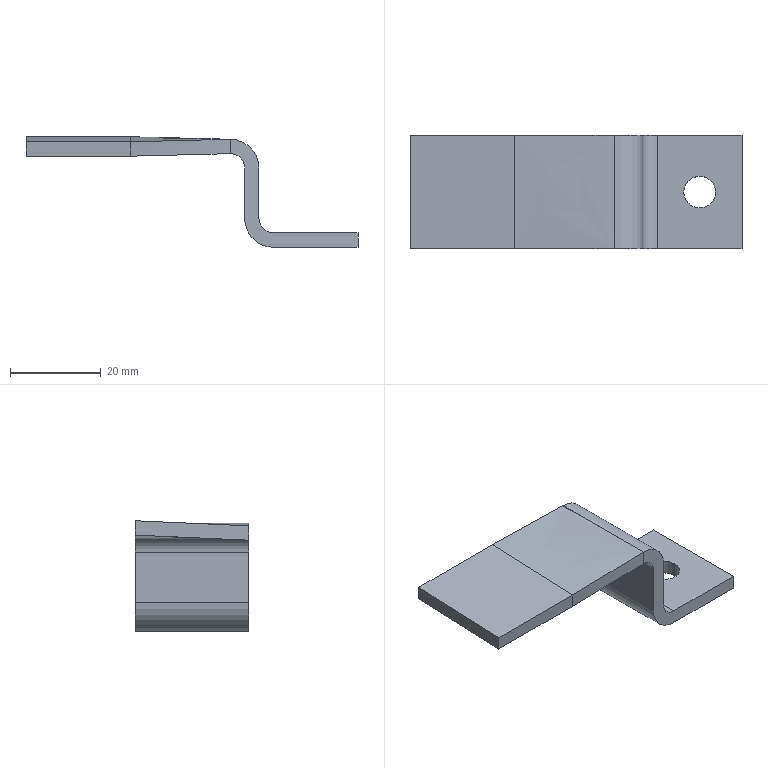Part | SolidWorks | features BaseBody 1 | 1 solid | 24 faces | box 73.18 x 25.116 x 24.356 mm | volume 6989 mm3 | plane 14 | cylinder 6 | spline 4 | commonest cylinder face diameters 6.34 x2 7 x2 12.68 x2
STEP:
#1=CARTESIAN_POINT('',(8.393,12.209,3.17));
#2=VERTEX_POINT('',#1);
#3=CARTESIAN_POINT('',(1.393,12.209,3.17));
#4=VERTEX_POINT('',#3);
#5=CARTESIAN_POINT('',(4.893,12.209,3.17));
#6=DIRECTION('',(0.,0.,-1.));
#7=DIRECTION('',(-1.,0.,0.));
#8=AXIS2_PLACEMENT_3D('',#5,#6,#7);
#9=CIRCLE('',#8,3.5);
#10=EDGE_CURVE('',#2,#4,#9,.T.);
#11=ORIENTED_EDGE('',*,*,#10,.F.);
#12=CARTESIAN_POINT('',(8.393,12.209,0.));
#13=VERTEX_POINT('',#12);
#14=CARTESIAN_POINT('',(8.393,12.209,81.122));
#15=DIRECTION('',(0.,0.,-1.));
#16=VECTOR('',#15,1000.);
#17=LINE('',#14,#16);
#18=EDGE_CURVE('',#2,#13,#17,.T.);
#19=ORIENTED_EDGE('',*,*,#18,.T.);
#20=CARTESIAN_POINT('',(1.393,12.209,0.));
#21=VERTEX_POINT('',#20);
#22=CARTESIAN_POINT('',(4.893,12.209,0.));
#23=DIRECTION('',(0.,0.,-1.));
#24=DIRECTION('',(-1.,0.,0.));
#25=AXIS2_PLACEMENT_3D('',#22,#23,#24);
#26=CIRCLE('',#25,3.5);
#27=EDGE_CURVE('',#13,#21,#26,.T.);
#28=ORIENTED_EDGE('',*,*,#27,.T.);
#29=CARTESIAN_POINT('',(1.393,12.209,81.122));
#30=DIRECTION('',(0.,0.,-1.));
#31=VECTOR('',#30,1000.);
#32=LINE('',#29,#31);
#33=EDGE_CURVE('',#4,#21,#32,.T.);
#34=ORIENTED_EDGE('',*,*,#33,.F.);
#35=EDGE_LOOP('',(#11,#19,#28,#34));
#36=FACE_OUTER_BOUND('',#35,.T.);
#37=CARTESIAN_POINT('',(4.893,12.209,81.122));
#38=DIRECTION('',(0.,0.,-1.));
#39=DIRECTION('',(-1.,0.,0.));
#40=AXIS2_PLACEMENT_3D('',#37,#38,#39);
#41=CYLINDRICAL_SURFACE('',#40,3.5);
#42=ADVANCED_FACE('',(#36),#41,.F.);
#43=CARTESIAN_POINT('',(-35.957,24.767,21.189));
#44=VERTEX_POINT('',#43);
#45=CARTESIAN_POINT('',(-35.957,-0.2082,20.074));
#46=VERTEX_POINT('',#45);
#47=CARTESIAN_POINT('',(-35.957,-0.2082,20.074));
#48=DIRECTION('',(0.,-0.999,-0.04458));
#49=VECTOR('',#48,1000.);
#50=LINE('',#47,#49);
#51=EDGE_CURVE('',#44,#46,#50,.T.);
#52=ORIENTED_EDGE('',*,*,#51,.T.);
#53=CARTESIAN_POINT('',(-58.957,-0.2082,20.074));
#54=VERTEX_POINT('',#53);
#55=CARTESIAN_POINT('',(-35.957,-0.2082,20.074));
#56=DIRECTION('',(-1.,0.,0.));
#57=VECTOR('',#56,1000.);
#58=LINE('',#55,#57);
#59=EDGE_CURVE('',#46,#54,#58,.T.);
#60=ORIENTED_EDGE('',*,*,#59,.T.);
#61=CARTESIAN_POINT('',(-58.957,24.767,21.189));
#62=VERTEX_POINT('',#61);
#63=CARTESIAN_POINT('',(-58.957,-0.2082,20.074));
#64=DIRECTION('',(0.,0.999,0.04458));
#65=VECTOR('',#64,1000.);
#66=LINE('',#63,#65);
#67=EDGE_CURVE('',#54,#62,#66,.T.);
#68=ORIENTED_EDGE('',*,*,#67,.T.);
#69=CARTESIAN_POINT('',(-35.957,24.767,21.189));
#70=DIRECTION('',(1.,0.,0.));
#71=VECTOR('',#70,1000.);
#72=LINE('',#69,#71);
#73=EDGE_CURVE('',#62,#44,#72,.T.);
#74=ORIENTED_EDGE('',*,*,#73,.T.);
#75=EDGE_LOOP('',(#52,#60,#68,#74));
#76=FACE_OUTER_BOUND('',#75,.T.);
#77=CARTESIAN_POINT('',(-35.957,-0.2082,20.074));
#78=DIRECTION('',(0.,0.04458,-0.999));
#79=DIRECTION('',(0.,0.999,0.04458));
#80=AXIS2_PLACEMENT_3D('',#77,#78,#79);
#81=PLANE('',#80);
#82=ADVANCED_FACE('',(#76),#81,.T.);
#83=CARTESIAN_POINT('',(-35.957,-0.3495,23.241));
#84=VERTEX_POINT('',#83);
#85=CARTESIAN_POINT('',(-35.957,-0.2788,21.658));
#86=DIRECTION('',(0.,0.04458,-0.999));
#87=VECTOR('',#86,1000.);
#88=LINE('',#85,#87);
#89=EDGE_CURVE('',#84,#46,#88,.T.);
#90=ORIENTED_EDGE('',*,*,#89,.F.);
#91=CARTESIAN_POINT('',(-58.957,-0.3495,23.241));
#92=VERTEX_POINT('',#91);
#93=CARTESIAN_POINT('',(-35.957,-0.3495,23.241));
#94=DIRECTION('',(-1.,0.,0.));
#95=VECTOR('',#94,1000.);
#96=LINE('',#93,#95);
#97=EDGE_CURVE('',#84,#92,#96,.T.);
#98=ORIENTED_EDGE('',*,*,#97,.T.);
#99=CARTESIAN_POINT('',(-58.957,-0.3495,23.241));
#100=DIRECTION('',(0.,0.04458,-0.999));
#101=VECTOR('',#100,1000.);
#102=LINE('',#99,#101);
#103=EDGE_CURVE('',#92,#54,#102,.T.);
#104=ORIENTED_EDGE('',*,*,#103,.T.);
#105=ORIENTED_EDGE('',*,*,#59,.F.);
#106=EDGE_LOOP('',(#90,#98,#104,#105));
#107=FACE_OUTER_BOUND('',#106,.T.);
#108=CARTESIAN_POINT('',(-35.957,-0.3495,23.241));
#109=DIRECTION('',(0.,-0.999,-0.04458));
#110=DIRECTION('',(0.,0.04458,-0.999));
#111=AXIS2_PLACEMENT_3D('',#108,#109,#110);
#112=PLANE('',#111);
#113=ADVANCED_FACE('',(#107),#112,.T.);
#114=CARTESIAN_POINT('',(-13.957,24.709,20.63));
#115=VERTEX_POINT('',#114);
#116=CARTESIAN_POINT('',(-13.957,-0.2913,20.63));
#117=VERTEX_POINT('',#116);
#118=CARTESIAN_POINT('',(-13.957,12.209,20.63));
#119=DIRECTION('',(0.,-1.,0.));
#120=VECTOR('',#119,1000.);
#121=LINE('',#118,#120);
#122=EDGE_CURVE('',#115,#117,#121,.T.);
#123=ORIENTED_EDGE('',*,*,#122,.T.);
#124=CARTESIAN_POINT('',(-13.957,-0.2913,20.63));
#125=CARTESIAN_POINT('',(-21.29,-0.2677,20.444));
#126=CARTESIAN_POINT('',(-28.623,-0.24,20.259));
#127=CARTESIAN_POINT('',(-35.957,-0.2082,20.074));
#128=B_SPLINE_CURVE_WITH_KNOTS('',3,(#124,#125,#126,#127),.UNSPECIFIED.,.F.,.F.,(4,4),(0.,0.04459),.UNSPECIFIED.);
#129=EDGE_CURVE('',#117,#46,#128,.T.);
#130=ORIENTED_EDGE('',*,*,#129,.T.);
#131=ORIENTED_EDGE('',*,*,#51,.F.);
#132=CARTESIAN_POINT('',(-35.957,24.767,21.189));
#133=CARTESIAN_POINT('',(-28.623,24.752,21.002));
#134=CARTESIAN_POINT('',(-21.29,24.732,20.816));
#135=CARTESIAN_POINT('',(-13.957,24.709,20.63));
#136=B_SPLINE_CURVE_WITH_KNOTS('',3,(#132,#133,#134,#135),.UNSPECIFIED.,.F.,.F.,(4,4),(0.,0.04459),.UNSPECIFIED.);
#137=EDGE_CURVE('',#44,#115,#136,.T.);
#138=ORIENTED_EDGE('',*,*,#137,.T.);
#139=EDGE_LOOP('',(#123,#130,#131,#138));
#140=FACE_OUTER_BOUND('',#139,.T.);
#141=CARTESIAN_POINT('',(-13.957,24.709,20.63));
#142=CARTESIAN_POINT('',(-21.29,24.732,20.816));
#143=CARTESIAN_POINT('',(-28.623,24.752,21.002));
#144=CARTESIAN_POINT('',(-35.957,24.767,21.189));
#145=CARTESIAN_POINT('',(-13.957,16.375,20.63));
#146=CARTESIAN_POINT('',(-21.29,16.399,20.692));
#147=CARTESIAN_POINT('',(-28.623,16.421,20.754));
#148=CARTESIAN_POINT('',(-35.957,16.442,20.817));
#149=CARTESIAN_POINT('',(-13.957,8.042,20.63));
#150=CARTESIAN_POINT('',(-21.29,8.066,20.568));
#151=CARTESIAN_POINT('',(-28.623,8.091,20.507));
#152=CARTESIAN_POINT('',(-35.957,8.117,20.446));
#153=CARTESIAN_POINT('',(-13.957,-0.2913,20.63));
#154=CARTESIAN_POINT('',(-21.29,-0.2677,20.444));
#155=CARTESIAN_POINT('',(-28.623,-0.24,20.259));
#156=CARTESIAN_POINT('',(-35.957,-0.2082,20.074));
#157=B_SPLINE_SURFACE_WITH_KNOTS('',3,3,((#141,#142,#143,#144),(#145,#146,#147,#148),(#149,#150,#151,#152),(#153,#154,#155,#156)),.UNSPECIFIED.,.F.,.F.,.F.,(4,4),(4,4),(0.,2.5),(0.,0.04459),.UNSPECIFIED.);
#158=ADVANCED_FACE('',(#140),#157,.T.);
#159=CARTESIAN_POINT('',(-35.957,24.626,24.356));
#160=VERTEX_POINT('',#159);
#161=CARTESIAN_POINT('',(-35.957,24.767,21.189));
#162=DIRECTION('',(0.,0.04458,-0.999));
#163=VECTOR('',#162,1000.);
#164=LINE('',#161,#163);
#165=EDGE_CURVE('',#160,#44,#164,.T.);
#166=ORIENTED_EDGE('',*,*,#165,.T.);
#167=ORIENTED_EDGE('',*,*,#73,.F.);
#168=CARTESIAN_POINT('',(-58.957,24.626,24.356));
#169=VERTEX_POINT('',#168);
#170=CARTESIAN_POINT('',(-58.957,24.767,21.189));
#171=DIRECTION('',(0.,-0.04458,0.999));
#172=VECTOR('',#171,1000.);
#173=LINE('',#170,#172);
#174=EDGE_CURVE('',#62,#169,#173,.T.);
#175=ORIENTED_EDGE('',*,*,#174,.T.);
#176=CARTESIAN_POINT('',(-35.957,24.626,24.356));
#177=DIRECTION('',(1.,0.,0.));
#178=VECTOR('',#177,1000.);
#179=LINE('',#176,#178);
#180=EDGE_CURVE('',#169,#160,#179,.T.);
#181=ORIENTED_EDGE('',*,*,#180,.T.);
#182=EDGE_LOOP('',(#166,#167,#175,#181));
#183=FACE_OUTER_BOUND('',#182,.T.);
#184=CARTESIAN_POINT('',(-35.957,24.767,21.189));
#185=DIRECTION('',(0.,0.999,0.04458));
#186=DIRECTION('',(0.,-0.04458,0.999));
#187=AXIS2_PLACEMENT_3D('',#184,#185,#186);
#188=PLANE('',#187);
#189=ADVANCED_FACE('',(#183),#188,.T.);
#190=CARTESIAN_POINT('',(-58.957,24.626,24.356));
#191=DIRECTION('',(0.,-0.999,-0.04458));
#192=VECTOR('',#191,1000.);
#193=LINE('',#190,#192);
#194=EDGE_CURVE('',#169,#92,#193,.T.);
#195=ORIENTED_EDGE('',*,*,#194,.F.);
#196=ORIENTED_EDGE('',*,*,#174,.F.);
#197=ORIENTED_EDGE('',*,*,#67,.F.);
#198=ORIENTED_EDGE('',*,*,#103,.F.);
#199=EDGE_LOOP('',(#195,#196,#197,#198));
#200=FACE_OUTER_BOUND('',#199,.T.);
#201=CARTESIAN_POINT('',(-58.957,12.209,22.215));
#202=DIRECTION('',(1.,0.,0.));
#203=DIRECTION('',(0.,1.,0.));
#204=AXIS2_PLACEMENT_3D('',#201,#202,#203);
#205=PLANE('',#204);
#206=ADVANCED_FACE('',(#200),#205,.F.);
#207=CARTESIAN_POINT('',(-35.957,24.626,24.356));
#208=DIRECTION('',(0.,0.999,0.04458));
#209=VECTOR('',#208,1000.);
#210=LINE('',#207,#209);
#211=EDGE_CURVE('',#84,#160,#210,.T.);
#212=ORIENTED_EDGE('',*,*,#211,.T.);
#213=ORIENTED_EDGE('',*,*,#180,.F.);
#214=ORIENTED_EDGE('',*,*,#194,.T.);
#215=ORIENTED_EDGE('',*,*,#97,.F.);
#216=EDGE_LOOP('',(#212,#213,#214,#215));
#217=FACE_OUTER_BOUND('',#216,.T.);
#218=CARTESIAN_POINT('',(-35.957,24.626,24.356));
#219=DIRECTION('',(0.,-0.04458,0.999));
#220=DIRECTION('',(0.,-0.999,-0.04458));
#221=AXIS2_PLACEMENT_3D('',#218,#219,#220);
#222=PLANE('',#221);
#223=ADVANCED_FACE('',(#217),#222,.T.);
#224=CARTESIAN_POINT('',(-13.957,-0.2913,23.8));
#225=VERTEX_POINT('',#224);
#226=CARTESIAN_POINT('',(-13.957,-0.2913,22.215));
#227=DIRECTION('',(0.,0.,1.));
#228=VECTOR('',#227,1000.);
#229=LINE('',#226,#228);
#230=EDGE_CURVE('',#117,#225,#229,.T.);
#231=ORIENTED_EDGE('',*,*,#230,.T.);
#232=CARTESIAN_POINT('',(-13.957,-0.2913,23.8));
#233=CARTESIAN_POINT('',(-21.29,-0.3148,23.614));
#234=CARTESIAN_POINT('',(-28.623,-0.3342,23.428));
#235=CARTESIAN_POINT('',(-35.957,-0.3495,23.241));
#236=B_SPLINE_CURVE_WITH_KNOTS('',3,(#232,#233,#234,#235),.UNSPECIFIED.,.F.,.F.,(4,4),(0.,0.04459),.UNSPECIFIED.);
#237=EDGE_CURVE('',#225,#84,#236,.T.);
#238=ORIENTED_EDGE('',*,*,#237,.T.);
#239=ORIENTED_EDGE('',*,*,#89,.T.);
#240=ORIENTED_EDGE('',*,*,#129,.F.);
#241=EDGE_LOOP('',(#231,#238,#239,#240));
#242=FACE_OUTER_BOUND('',#241,.T.);
#243=CARTESIAN_POINT('',(-13.957,-0.2913,20.63));
#244=CARTESIAN_POINT('',(-21.29,-0.2677,20.444));
#245=CARTESIAN_POINT('',(-28.623,-0.24,20.259));
#246=CARTESIAN_POINT('',(-35.957,-0.2082,20.074));
#247=CARTESIAN_POINT('',(-13.957,-0.2913,21.687));
#248=CARTESIAN_POINT('',(-21.29,-0.2834,21.501));
#249=CARTESIAN_POINT('',(-28.623,-0.2714,21.315));
#250=CARTESIAN_POINT('',(-35.957,-0.2553,21.13));
#251=CARTESIAN_POINT('',(-13.957,-0.2913,22.743));
#252=CARTESIAN_POINT('',(-21.29,-0.2991,22.558));
#253=CARTESIAN_POINT('',(-28.623,-0.3028,22.372));
#254=CARTESIAN_POINT('',(-35.957,-0.3024,22.186));
#255=CARTESIAN_POINT('',(-13.957,-0.2913,23.8));
#256=CARTESIAN_POINT('',(-21.29,-0.3148,23.614));
#257=CARTESIAN_POINT('',(-28.623,-0.3342,23.428));
#258=CARTESIAN_POINT('',(-35.957,-0.3495,23.241));
#259=B_SPLINE_SURFACE_WITH_KNOTS('',3,3,((#243,#244,#245,#246),(#247,#248,#249,#250),(#251,#252,#253,#254),(#255,#256,#257,#258)),.UNSPECIFIED.,.F.,.F.,.F.,(4,4),(4,4),(0.,0.317),(0.,0.04459),.UNSPECIFIED.);
#260=ADVANCED_FACE('',(#242),#259,.T.);
#261=ORIENTED_EDGE('',*,*,#122,.F.);
#262=CARTESIAN_POINT('',(-13.947,24.709,20.63));
#263=VERTEX_POINT('',#262);
#264=CARTESIAN_POINT('',(-10.782,24.709,20.63));
#265=DIRECTION('',(-1.,0.,0.));
#266=VECTOR('',#265,1000.);
#267=LINE('',#264,#266);
#268=EDGE_CURVE('',#263,#115,#267,.T.);
#269=ORIENTED_EDGE('',*,*,#268,.F.);
#270=CARTESIAN_POINT('',(-13.947,-0.2913,20.63));
#271=VERTEX_POINT('',#270);
#272=CARTESIAN_POINT('',(-13.947,-0.2913,20.63));
#273=DIRECTION('',(0.,-1.,0.));
#274=VECTOR('',#273,1000.);
#275=LINE('',#272,#274);
#276=EDGE_CURVE('',#263,#271,#275,.T.);
#277=ORIENTED_EDGE('',*,*,#276,.T.);
#278=CARTESIAN_POINT('',(-10.782,-0.2913,20.63));
#279=DIRECTION('',(-1.,0.,0.));
#280=VECTOR('',#279,1000.);
#281=LINE('',#278,#280);
#282=EDGE_CURVE('',#271,#117,#281,.T.);
#283=ORIENTED_EDGE('',*,*,#282,.T.);
#284=EDGE_LOOP('',(#261,#269,#277,#283));
#285=FACE_OUTER_BOUND('',#284,.T.);
#286=CARTESIAN_POINT('',(-13.957,-0.2913,20.63));
#287=DIRECTION('',(0.,0.,-1.));
#288=DIRECTION('',(-1.,0.,0.));
#289=AXIS2_PLACEMENT_3D('',#286,#287,#288);
#290=PLANE('',#289);
#291=ADVANCED_FACE('',(#285),#290,.T.);
#292=CARTESIAN_POINT('',(-13.957,24.709,23.8));
#293=VERTEX_POINT('',#292);
#294=CARTESIAN_POINT('',(-13.957,24.709,22.215));
#295=DIRECTION('',(0.,0.,1.));
#296=VECTOR('',#295,1000.);
#297=LINE('',#294,#296);
#298=EDGE_CURVE('',#115,#293,#297,.T.);
#299=ORIENTED_EDGE('',*,*,#298,.F.);
#300=ORIENTED_EDGE('',*,*,#137,.F.);
#301=ORIENTED_EDGE('',*,*,#165,.F.);
#302=CARTESIAN_POINT('',(-35.957,24.626,24.356));
#303=CARTESIAN_POINT('',(-28.623,24.657,24.171));
#304=CARTESIAN_POINT('',(-21.29,24.685,23.986));
#305=CARTESIAN_POINT('',(-13.957,24.709,23.8));
#306=B_SPLINE_CURVE_WITH_KNOTS('',3,(#302,#303,#304,#305),.UNSPECIFIED.,.F.,.F.,(4,4),(0.,0.04459),.UNSPECIFIED.);
#307=EDGE_CURVE('',#160,#293,#306,.T.);
#308=ORIENTED_EDGE('',*,*,#307,.T.);
#309=EDGE_LOOP('',(#299,#300,#301,#308));
#310=FACE_OUTER_BOUND('',#309,.T.);
#311=CARTESIAN_POINT('',(-13.957,24.709,23.8));
#312=CARTESIAN_POINT('',(-21.29,24.685,23.986));
#313=CARTESIAN_POINT('',(-28.623,24.657,24.171));
#314=CARTESIAN_POINT('',(-35.957,24.626,24.356));
#315=CARTESIAN_POINT('',(-13.957,24.709,22.743));
#316=CARTESIAN_POINT('',(-21.29,24.701,22.929));
#317=CARTESIAN_POINT('',(-28.623,24.689,23.115));
#318=CARTESIAN_POINT('',(-35.957,24.673,23.3));
#319=CARTESIAN_POINT('',(-13.957,24.709,21.687));
#320=CARTESIAN_POINT('',(-21.29,24.717,21.872));
#321=CARTESIAN_POINT('',(-28.623,24.72,22.058));
#322=CARTESIAN_POINT('',(-35.957,24.72,22.244));
#323=CARTESIAN_POINT('',(-13.957,24.709,20.63));
#324=CARTESIAN_POINT('',(-21.29,24.732,20.816));
#325=CARTESIAN_POINT('',(-28.623,24.752,21.002));
#326=CARTESIAN_POINT('',(-35.957,24.767,21.189));
#327=B_SPLINE_SURFACE_WITH_KNOTS('',3,3,((#311,#312,#313,#314),(#315,#316,#317,#318),(#319,#320,#321,#322),(#323,#324,#325,#326)),.UNSPECIFIED.,.F.,.F.,.F.,(4,4),(4,4),(0.,0.317),(0.,0.04459),.UNSPECIFIED.);
#328=ADVANCED_FACE('',(#310),#327,.T.);
#329=CARTESIAN_POINT('',(-13.957,12.209,23.8));
#330=DIRECTION('',(0.,1.,0.));
#331=VECTOR('',#330,1000.);
#332=LINE('',#329,#331);
#333=EDGE_CURVE('',#225,#293,#332,.T.);
#334=ORIENTED_EDGE('',*,*,#333,.T.);
#335=ORIENTED_EDGE('',*,*,#307,.F.);
#336=ORIENTED_EDGE('',*,*,#211,.F.);
#337=ORIENTED_EDGE('',*,*,#237,.F.);
#338=EDGE_LOOP('',(#334,#335,#336,#337));
#339=FACE_OUTER_BOUND('',#338,.T.);
#340=CARTESIAN_POINT('',(-13.957,-0.2913,23.8));
#341=CARTESIAN_POINT('',(-21.29,-0.3148,23.614));
#342=CARTESIAN_POINT('',(-28.623,-0.3342,23.428));
#343=CARTESIAN_POINT('',(-35.957,-0.3495,23.241));
#344=CARTESIAN_POINT('',(-13.957,8.042,23.8));
#345=CARTESIAN_POINT('',(-21.29,8.019,23.738));
#346=CARTESIAN_POINT('',(-28.623,7.996,23.676));
#347=CARTESIAN_POINT('',(-35.957,7.976,23.613));
#348=CARTESIAN_POINT('',(-13.957,16.375,23.8));
#349=CARTESIAN_POINT('',(-21.29,16.352,23.862));
#350=CARTESIAN_POINT('',(-28.623,16.327,23.923));
#351=CARTESIAN_POINT('',(-35.957,16.301,23.984));
#352=CARTESIAN_POINT('',(-13.957,24.709,23.8));
#353=CARTESIAN_POINT('',(-21.29,24.685,23.986));
#354=CARTESIAN_POINT('',(-28.623,24.657,24.171));
#355=CARTESIAN_POINT('',(-35.957,24.626,24.356));
#356=B_SPLINE_SURFACE_WITH_KNOTS('',3,3,((#340,#341,#342,#343),(#344,#345,#346,#347),(#348,#349,#350,#351),(#352,#353,#354,#355)),.UNSPECIFIED.,.F.,.F.,.F.,(4,4),(4,4),(0.,2.5),(0.,0.04459),.UNSPECIFIED.);
#357=ADVANCED_FACE('',(#339),#356,.T.);
#358=CARTESIAN_POINT('',(-10.777,24.709,17.46));
#359=VERTEX_POINT('',#358);
#360=CARTESIAN_POINT('',(-13.947,24.709,17.46));
#361=DIRECTION('',(0.,-1.,0.));
#362=DIRECTION('',(1.,0.,0.));
#363=AXIS2_PLACEMENT_3D('',#360,#361,#362);
#364=CIRCLE('',#363,3.17);
#365=EDGE_CURVE('',#359,#263,#364,.T.);
#366=ORIENTED_EDGE('',*,*,#365,.F.);
#367=CARTESIAN_POINT('',(-10.777,-0.2913,17.46));
#368=VERTEX_POINT('',#367);
#369=CARTESIAN_POINT('',(-10.777,12.209,17.46));
#370=DIRECTION('',(0.,1.,0.));
#371=VECTOR('',#370,1000.);
#372=LINE('',#369,#371);
#373=EDGE_CURVE('',#368,#359,#372,.T.);
#374=ORIENTED_EDGE('',*,*,#373,.F.);
#375=CARTESIAN_POINT('',(-13.947,-0.2913,17.46));
#376=DIRECTION('',(0.,1.,0.));
#377=DIRECTION('',(1.,0.,0.));
#378=AXIS2_PLACEMENT_3D('',#375,#376,#377);
#379=CIRCLE('',#378,3.17);
#380=EDGE_CURVE('',#271,#368,#379,.T.);
#381=ORIENTED_EDGE('',*,*,#380,.F.);
#382=ORIENTED_EDGE('',*,*,#276,.F.);
#383=EDGE_LOOP('',(#366,#374,#381,#382));
#384=FACE_OUTER_BOUND('',#383,.T.);
#385=CARTESIAN_POINT('',(-13.947,12.209,17.46));
#386=DIRECTION('',(0.,-1.,0.));
#387=DIRECTION('',(1.,0.,0.));
#388=AXIS2_PLACEMENT_3D('',#385,#386,#387);
#389=CYLINDRICAL_SURFACE('',#388,3.17);
#390=ADVANCED_FACE('',(#384),#389,.F.);
#391=ORIENTED_EDGE('',*,*,#333,.F.);
#392=CARTESIAN_POINT('',(-13.947,-0.2913,23.8));
#393=VERTEX_POINT('',#392);
#394=CARTESIAN_POINT('',(-7.607,-0.2913,23.8));
#395=DIRECTION('',(1.,0.,0.));
#396=VECTOR('',#395,1000.);
#397=LINE('',#394,#396);
#398=EDGE_CURVE('',#225,#393,#397,.T.);
#399=ORIENTED_EDGE('',*,*,#398,.T.);
#400=CARTESIAN_POINT('',(-13.947,24.709,23.8));
#401=VERTEX_POINT('',#400);
#402=CARTESIAN_POINT('',(-13.947,-0.2913,23.8));
#403=DIRECTION('',(0.,1.,0.));
#404=VECTOR('',#403,1000.);
#405=LINE('',#402,#404);
#406=EDGE_CURVE('',#393,#401,#405,.T.);
#407=ORIENTED_EDGE('',*,*,#406,.T.);
#408=CARTESIAN_POINT('',(-7.607,24.709,23.8));
#409=DIRECTION('',(-1.,0.,0.));
#410=VECTOR('',#409,1000.);
#411=LINE('',#408,#410);
#412=EDGE_CURVE('',#401,#293,#411,.T.);
#413=ORIENTED_EDGE('',*,*,#412,.T.);
#414=EDGE_LOOP('',(#391,#399,#407,#413));
#415=FACE_OUTER_BOUND('',#414,.T.);
#416=CARTESIAN_POINT('',(-7.607,-0.2913,23.8));
#417=DIRECTION('',(0.,0.,1.));
#418=DIRECTION('',(1.,0.,0.));
#419=AXIS2_PLACEMENT_3D('',#416,#417,#418);
#420=PLANE('',#419);
#421=ADVANCED_FACE('',(#415),#420,.T.);
#422=CARTESIAN_POINT('',(-10.777,24.709,6.34));
#423=VERTEX_POINT('',#422);
#424=CARTESIAN_POINT('',(-10.777,24.709,22.215));
#425=DIRECTION('',(0.,0.,1.));
#426=VECTOR('',#425,1000.);
#427=LINE('',#424,#426);
#428=EDGE_CURVE('',#423,#359,#427,.T.);
#429=ORIENTED_EDGE('',*,*,#428,.T.);
#430=ORIENTED_EDGE('',*,*,#365,.T.);
#431=ORIENTED_EDGE('',*,*,#268,.T.);
#432=ORIENTED_EDGE('',*,*,#298,.T.);
#433=ORIENTED_EDGE('',*,*,#412,.F.);
#434=CARTESIAN_POINT('',(-7.607,24.709,17.46));
#435=VERTEX_POINT('',#434);
#436=CARTESIAN_POINT('',(-13.947,24.709,17.46));
#437=DIRECTION('',(0.,1.,0.));
#438=DIRECTION('',(1.,0.,0.));
#439=AXIS2_PLACEMENT_3D('',#436,#437,#438);
#440=CIRCLE('',#439,6.34);
#441=EDGE_CURVE('',#401,#435,#440,.T.);
#442=ORIENTED_EDGE('',*,*,#441,.T.);
#443=CARTESIAN_POINT('',(-7.607,24.709,6.34));
#444=VERTEX_POINT('',#443);
#445=CARTESIAN_POINT('',(-7.607,24.709,22.215));
#446=DIRECTION('',(0.,0.,-1.));
#447=VECTOR('',#446,1000.);
#448=LINE('',#445,#447);
#449=EDGE_CURVE('',#435,#444,#448,.T.);
#450=ORIENTED_EDGE('',*,*,#449,.T.);
#451=CARTESIAN_POINT('',(-4.437,24.709,3.17));
#452=VERTEX_POINT('',#451);
#453=CARTESIAN_POINT('',(-4.437,24.709,6.34));
#454=DIRECTION('',(0.,-1.,0.));
#455=DIRECTION('',(-1.,0.,0.));
#456=AXIS2_PLACEMENT_3D('',#453,#454,#455);
#457=CIRCLE('',#456,3.17);
#458=EDGE_CURVE('',#444,#452,#457,.T.);
#459=ORIENTED_EDGE('',*,*,#458,.T.);
#460=CARTESIAN_POINT('',(14.223,24.709,3.17));
#461=VERTEX_POINT('',#460);
#462=CARTESIAN_POINT('',(-10.782,24.709,3.17));
#463=DIRECTION('',(1.,0.,0.));
#464=VECTOR('',#463,1000.);
#465=LINE('',#462,#464);
#466=EDGE_CURVE('',#452,#461,#465,.T.);
#467=ORIENTED_EDGE('',*,*,#466,.T.);
#468=CARTESIAN_POINT('',(14.223,24.709,0.));
#469=VERTEX_POINT('',#468);
#470=CARTESIAN_POINT('',(14.223,24.709,22.215));
#471=DIRECTION('',(0.,0.,-1.));
#472=VECTOR('',#471,1000.);
#473=LINE('',#470,#472);
#474=EDGE_CURVE('',#461,#469,#473,.T.);
#475=ORIENTED_EDGE('',*,*,#474,.T.);
#476=CARTESIAN_POINT('',(-4.437,24.709,0.));
#477=VERTEX_POINT('',#476);
#478=CARTESIAN_POINT('',(-10.782,24.709,0.));
#479=DIRECTION('',(-1.,0.,0.));
#480=VECTOR('',#479,1000.);
#481=LINE('',#478,#480);
#482=EDGE_CURVE('',#469,#477,#481,.T.);
#483=ORIENTED_EDGE('',*,*,#482,.T.);
#484=CARTESIAN_POINT('',(-4.437,24.709,6.34));
#485=DIRECTION('',(0.,1.,0.));
#486=DIRECTION('',(-1.,0.,0.));
#487=AXIS2_PLACEMENT_3D('',#484,#485,#486);
#488=CIRCLE('',#487,6.34);
#489=EDGE_CURVE('',#477,#423,#488,.T.);
#490=ORIENTED_EDGE('',*,*,#489,.T.);
#491=EDGE_LOOP('',(#429,#430,#431,#432,#433,#442,#450,#459,#467,#475,#483,#490));
#492=FACE_OUTER_BOUND('',#491,.T.);
#493=CARTESIAN_POINT('',(-10.782,24.709,22.215));
#494=DIRECTION('',(0.,1.,0.));
#495=DIRECTION('',(-1.,0.,0.));
#496=AXIS2_PLACEMENT_3D('',#493,#494,#495);
#497=PLANE('',#496);
#498=ADVANCED_FACE('',(#492),#497,.T.);
#499=CARTESIAN_POINT('',(-10.777,-0.2913,6.34));
#500=VERTEX_POINT('',#499);
#501=CARTESIAN_POINT('',(-10.777,24.709,6.34));
#502=DIRECTION('',(0.,-1.,0.));
#503=VECTOR('',#502,1000.);
#504=LINE('',#501,#503);
#505=EDGE_CURVE('',#423,#500,#504,.T.);
#506=ORIENTED_EDGE('',*,*,#505,.T.);
#507=CARTESIAN_POINT('',(-10.777,-0.2913,0.));
#508=DIRECTION('',(0.,0.,1.));
#509=VECTOR('',#508,1000.);
#510=LINE('',#507,#509);
#511=EDGE_CURVE('',#500,#368,#510,.T.);
#512=ORIENTED_EDGE('',*,*,#511,.T.);
#513=ORIENTED_EDGE('',*,*,#373,.T.);
#514=ORIENTED_EDGE('',*,*,#428,.F.);
#515=EDGE_LOOP('',(#506,#512,#513,#514));
#516=FACE_OUTER_BOUND('',#515,.T.);
#517=CARTESIAN_POINT('',(-10.777,24.709,0.));
#518=DIRECTION('',(-1.,0.,0.));
#519=DIRECTION('',(0.,-1.,0.));
#520=AXIS2_PLACEMENT_3D('',#517,#518,#519);
#521=PLANE('',#520);
#522=ADVANCED_FACE('',(#516),#521,.T.);
#523=ORIENTED_EDGE('',*,*,#230,.F.);
#524=ORIENTED_EDGE('',*,*,#282,.F.);
#525=ORIENTED_EDGE('',*,*,#380,.T.);
#526=ORIENTED_EDGE('',*,*,#511,.F.);
#527=CARTESIAN_POINT('',(-4.437,-0.2913,0.));
#528=VERTEX_POINT('',#527);
#529=CARTESIAN_POINT('',(-4.437,-0.2913,6.34));
#530=DIRECTION('',(0.,1.,0.));
#531=DIRECTION('',(-1.,0.,0.));
#532=AXIS2_PLACEMENT_3D('',#529,#530,#531);
#533=CIRCLE('',#532,6.34);
#534=EDGE_CURVE('',#528,#500,#533,.T.);
#535=ORIENTED_EDGE('',*,*,#534,.F.);
#536=CARTESIAN_POINT('',(14.223,-0.2913,0.));
#537=VERTEX_POINT('',#536);
#538=CARTESIAN_POINT('',(-10.782,-0.2913,0.));
#539=DIRECTION('',(-1.,0.,0.));
#540=VECTOR('',#539,1000.);
#541=LINE('',#538,#540);
#542=EDGE_CURVE('',#537,#528,#541,.T.);
#543=ORIENTED_EDGE('',*,*,#542,.F.);
#544=CARTESIAN_POINT('',(14.223,-0.2913,3.17));
#545=VERTEX_POINT('',#544);
#546=CARTESIAN_POINT('',(14.223,-0.2913,22.215));
#547=DIRECTION('',(0.,0.,-1.));
#548=VECTOR('',#547,1000.);
#549=LINE('',#546,#548);
#550=EDGE_CURVE('',#545,#537,#549,.T.);
#551=ORIENTED_EDGE('',*,*,#550,.F.);
#552=CARTESIAN_POINT('',(-4.437,-0.2913,3.17));
#553=VERTEX_POINT('',#552);
#554=CARTESIAN_POINT('',(-10.782,-0.2913,3.17));
#555=DIRECTION('',(1.,0.,0.));
#556=VECTOR('',#555,1000.);
#557=LINE('',#554,#556);
#558=EDGE_CURVE('',#553,#545,#557,.T.);
#559=ORIENTED_EDGE('',*,*,#558,.F.);
#560=CARTESIAN_POINT('',(-7.607,-0.2913,6.34));
#561=VERTEX_POINT('',#560);
#562=CARTESIAN_POINT('',(-4.437,-0.2913,6.34));
#563=DIRECTION('',(0.,-1.,0.));
#564=DIRECTION('',(-1.,0.,0.));
#565=AXIS2_PLACEMENT_3D('',#562,#563,#564);
#566=CIRCLE('',#565,3.17);
#567=EDGE_CURVE('',#561,#553,#566,.T.);
#568=ORIENTED_EDGE('',*,*,#567,.F.);
#569=CARTESIAN_POINT('',(-7.607,-0.2913,17.46));
#570=VERTEX_POINT('',#569);
#571=CARTESIAN_POINT('',(-7.607,-0.2913,22.215));
#572=DIRECTION('',(0.,0.,-1.));
#573=VECTOR('',#572,1000.);
#574=LINE('',#571,#573);
#575=EDGE_CURVE('',#570,#561,#574,.T.);
#576=ORIENTED_EDGE('',*,*,#575,.F.);
#577=CARTESIAN_POINT('',(-13.947,-0.2913,17.46));
#578=DIRECTION('',(0.,1.,0.));
#579=DIRECTION('',(1.,0.,0.));
#580=AXIS2_PLACEMENT_3D('',#577,#578,#579);
#581=CIRCLE('',#580,6.34);
#582=EDGE_CURVE('',#393,#570,#581,.T.);
#583=ORIENTED_EDGE('',*,*,#582,.F.);
#584=ORIENTED_EDGE('',*,*,#398,.F.);
#585=EDGE_LOOP('',(#523,#524,#525,#526,#535,#543,#551,#559,#568,#576,#583,#584));
#586=FACE_OUTER_BOUND('',#585,.T.);
#587=CARTESIAN_POINT('',(-10.782,-0.2913,22.215));
#588=DIRECTION('',(0.,1.,0.));
#589=DIRECTION('',(-1.,0.,0.));
#590=AXIS2_PLACEMENT_3D('',#587,#588,#589);
#591=PLANE('',#590);
#592=ADVANCED_FACE('',(#586),#591,.F.);
#593=CARTESIAN_POINT('',(-7.607,12.209,17.46));
#594=DIRECTION('',(0.,1.,0.));
#595=VECTOR('',#594,1000.);
#596=LINE('',#593,#595);
#597=EDGE_CURVE('',#570,#435,#596,.T.);
#598=ORIENTED_EDGE('',*,*,#597,.T.);
#599=ORIENTED_EDGE('',*,*,#441,.F.);
#600=ORIENTED_EDGE('',*,*,#406,.F.);
#601=ORIENTED_EDGE('',*,*,#582,.T.);
#602=EDGE_LOOP('',(#598,#599,#600,#601));
#603=FACE_OUTER_BOUND('',#602,.T.);
#604=CARTESIAN_POINT('',(-13.947,12.209,17.46));
#605=DIRECTION('',(0.,-1.,0.));
#606=DIRECTION('',(1.,0.,0.));
#607=AXIS2_PLACEMENT_3D('',#604,#605,#606);
#608=CYLINDRICAL_SURFACE('',#607,6.34);
#609=ADVANCED_FACE('',(#603),#608,.T.);
#610=CARTESIAN_POINT('',(-4.437,12.209,0.));
#611=DIRECTION('',(0.,-1.,0.));
#612=VECTOR('',#611,1000.);
#613=LINE('',#610,#612);
#614=EDGE_CURVE('',#477,#528,#613,.T.);
#615=ORIENTED_EDGE('',*,*,#614,.T.);
#616=ORIENTED_EDGE('',*,*,#534,.T.);
#617=ORIENTED_EDGE('',*,*,#505,.F.);
#618=ORIENTED_EDGE('',*,*,#489,.F.);
#619=EDGE_LOOP('',(#615,#616,#617,#618));
#620=FACE_OUTER_BOUND('',#619,.T.);
#621=CARTESIAN_POINT('',(-4.437,12.209,6.34));
#622=DIRECTION('',(0.,1.,0.));
#623=DIRECTION('',(-1.,0.,0.));
#624=AXIS2_PLACEMENT_3D('',#621,#622,#623);
#625=CYLINDRICAL_SURFACE('',#624,6.34);
#626=ADVANCED_FACE('',(#620),#625,.T.);
#627=CARTESIAN_POINT('',(4.893,12.209,0.));
#628=DIRECTION('',(0.,0.,-1.));
#629=DIRECTION('',(-1.,0.,0.));
#630=AXIS2_PLACEMENT_3D('',#627,#628,#629);
#631=CIRCLE('',#630,3.5);
#632=EDGE_CURVE('',#21,#13,#631,.T.);
#633=ORIENTED_EDGE('',*,*,#632,.F.);
#634=ORIENTED_EDGE('',*,*,#27,.F.);
#635=EDGE_LOOP('',(#633,#634));
#636=FACE_BOUND('',#635,.T.);
#637=ORIENTED_EDGE('',*,*,#482,.F.);
#638=CARTESIAN_POINT('',(14.223,12.209,0.));
#639=DIRECTION('',(0.,1.,0.));
#640=VECTOR('',#639,1000.);
#641=LINE('',#638,#640);
#642=EDGE_CURVE('',#537,#469,#641,.T.);
#643=ORIENTED_EDGE('',*,*,#642,.F.);
#644=ORIENTED_EDGE('',*,*,#542,.T.);
#645=ORIENTED_EDGE('',*,*,#614,.F.);
#646=EDGE_LOOP('',(#637,#643,#644,#645));
#647=FACE_OUTER_BOUND('',#646,.T.);
#648=CARTESIAN_POINT('',(1.723,12.209,0.));
#649=DIRECTION('',(0.,0.,1.));
#650=DIRECTION('',(1.,0.,0.));
#651=AXIS2_PLACEMENT_3D('',#648,#649,#650);
#652=PLANE('',#651);
#653=ADVANCED_FACE('',(#636,#647),#652,.F.);
#654=ORIENTED_EDGE('',*,*,#642,.T.);
#655=ORIENTED_EDGE('',*,*,#474,.F.);
#656=CARTESIAN_POINT('',(14.223,24.709,3.17));
#657=DIRECTION('',(0.,-1.,0.));
#658=VECTOR('',#657,1000.);
#659=LINE('',#656,#658);
#660=EDGE_CURVE('',#461,#545,#659,.T.);
#661=ORIENTED_EDGE('',*,*,#660,.T.);
#662=ORIENTED_EDGE('',*,*,#550,.T.);
#663=EDGE_LOOP('',(#654,#655,#661,#662));
#664=FACE_OUTER_BOUND('',#663,.T.);
#665=CARTESIAN_POINT('',(14.223,24.709,0.));
#666=DIRECTION('',(1.,0.,0.));
#667=DIRECTION('',(0.,1.,0.));
#668=AXIS2_PLACEMENT_3D('',#665,#666,#667);
#669=PLANE('',#668);
#670=ADVANCED_FACE('',(#664),#669,.T.);
#671=CARTESIAN_POINT('',(4.893,12.209,3.17));
#672=DIRECTION('',(0.,0.,-1.));
#673=DIRECTION('',(-1.,0.,0.));
#674=AXIS2_PLACEMENT_3D('',#671,#672,#673);
#675=CIRCLE('',#674,3.5);
#676=EDGE_CURVE('',#4,#2,#675,.T.);
#677=ORIENTED_EDGE('',*,*,#676,.T.);
#678=ORIENTED_EDGE('',*,*,#10,.T.);
#679=EDGE_LOOP('',(#677,#678));
#680=FACE_BOUND('',#679,.T.);
#681=ORIENTED_EDGE('',*,*,#660,.F.);
#682=ORIENTED_EDGE('',*,*,#466,.F.);
#683=CARTESIAN_POINT('',(-4.437,12.209,3.17));
#684=DIRECTION('',(0.,-1.,0.));
#685=VECTOR('',#684,1000.);
#686=LINE('',#683,#685);
#687=EDGE_CURVE('',#452,#553,#686,.T.);
#688=ORIENTED_EDGE('',*,*,#687,.T.);
#689=ORIENTED_EDGE('',*,*,#558,.T.);
#690=EDGE_LOOP('',(#681,#682,#688,#689));
#691=FACE_OUTER_BOUND('',#690,.T.);
#692=CARTESIAN_POINT('',(1.723,12.209,3.17));
#693=DIRECTION('',(0.,0.,1.));
#694=DIRECTION('',(1.,0.,0.));
#695=AXIS2_PLACEMENT_3D('',#692,#693,#694);
#696=PLANE('',#695);
#697=ADVANCED_FACE('',(#680,#691),#696,.T.);
#698=ORIENTED_EDGE('',*,*,#567,.T.);
#699=ORIENTED_EDGE('',*,*,#687,.F.);
#700=ORIENTED_EDGE('',*,*,#458,.F.);
#701=CARTESIAN_POINT('',(-7.607,12.209,6.34));
#702=DIRECTION('',(0.,1.,0.));
#703=VECTOR('',#702,1000.);
#704=LINE('',#701,#703);
#705=EDGE_CURVE('',#561,#444,#704,.T.);
#706=ORIENTED_EDGE('',*,*,#705,.F.);
#707=EDGE_LOOP('',(#698,#699,#700,#706));
#708=FACE_OUTER_BOUND('',#707,.T.);
#709=CARTESIAN_POINT('',(-4.437,12.209,6.34));
#710=DIRECTION('',(0.,1.,0.));
#711=DIRECTION('',(-1.,0.,0.));
#712=AXIS2_PLACEMENT_3D('',#709,#710,#711);
#713=CYLINDRICAL_SURFACE('',#712,3.17);
#714=ADVANCED_FACE('',(#708),#713,.F.);
#715=ORIENTED_EDGE('',*,*,#705,.T.);
#716=ORIENTED_EDGE('',*,*,#449,.F.);
#717=ORIENTED_EDGE('',*,*,#597,.F.);
#718=ORIENTED_EDGE('',*,*,#575,.T.);
#719=EDGE_LOOP('',(#715,#716,#717,#718));
#720=FACE_OUTER_BOUND('',#719,.T.);
#721=CARTESIAN_POINT('',(-7.607,24.709,23.8));
#722=DIRECTION('',(1.,0.,0.));
#723=DIRECTION('',(0.,1.,0.));
#724=AXIS2_PLACEMENT_3D('',#721,#722,#723);
#725=PLANE('',#724);
#726=ADVANCED_FACE('',(#720),#725,.T.);
#727=ORIENTED_EDGE('',*,*,#18,.F.);
#728=ORIENTED_EDGE('',*,*,#676,.F.);
#729=ORIENTED_EDGE('',*,*,#33,.T.);
#730=ORIENTED_EDGE('',*,*,#632,.T.);
#731=EDGE_LOOP('',(#727,#728,#729,#730));
#732=FACE_OUTER_BOUND('',#731,.T.);
#733=CARTESIAN_POINT('',(4.893,12.209,81.122));
#734=DIRECTION('',(0.,0.,-1.));
#735=DIRECTION('',(-1.,0.,0.));
#736=AXIS2_PLACEMENT_3D('',#733,#734,#735);
#737=CYLINDRICAL_SURFACE('',#736,3.5);
#738=ADVANCED_FACE('',(#732),#737,.F.);
#739=CLOSED_SHELL('',(#42,#82,#113,#158,#189,#206,#223,#260,#291,#328,#357,#390,#421,#498,#522,#592,#609,#626,#653,#670,#697,#714,#726,#738));
#740=MANIFOLD_SOLID_BREP('',#739);
#741=CARTESIAN_POINT('',(0.,0.,0.));
#742=DIRECTION('',(0.,0.,1.));
#743=DIRECTION('',(1.,0.,0.));
#744=AXIS2_PLACEMENT_3D('',#741,#742,#743);
#745=(LENGTH_UNIT()NAMED_UNIT(*)SI_UNIT(.MILLI.,.METRE.));
#746=UNCERTAINTY_MEASURE_WITH_UNIT(LENGTH_MEASURE(0.00001),#745,'','');
#747=(NAMED_UNIT(*)PLANE_ANGLE_UNIT()SI_UNIT($,.RADIAN.));
#748=(NAMED_UNIT(*)SI_UNIT($,.STERADIAN.)SOLID_ANGLE_UNIT());
#749=(GEOMETRIC_REPRESENTATION_CONTEXT(3)GLOBAL_UNCERTAINTY_ASSIGNED_CONTEXT((#746))GLOBAL_UNIT_ASSIGNED_CONTEXT((#745,#747,#748))REPRESENTATION_CONTEXT('',''));
#750=ADVANCED_BREP_SHAPE_REPRESENTATION('',(#740,#744),#749);